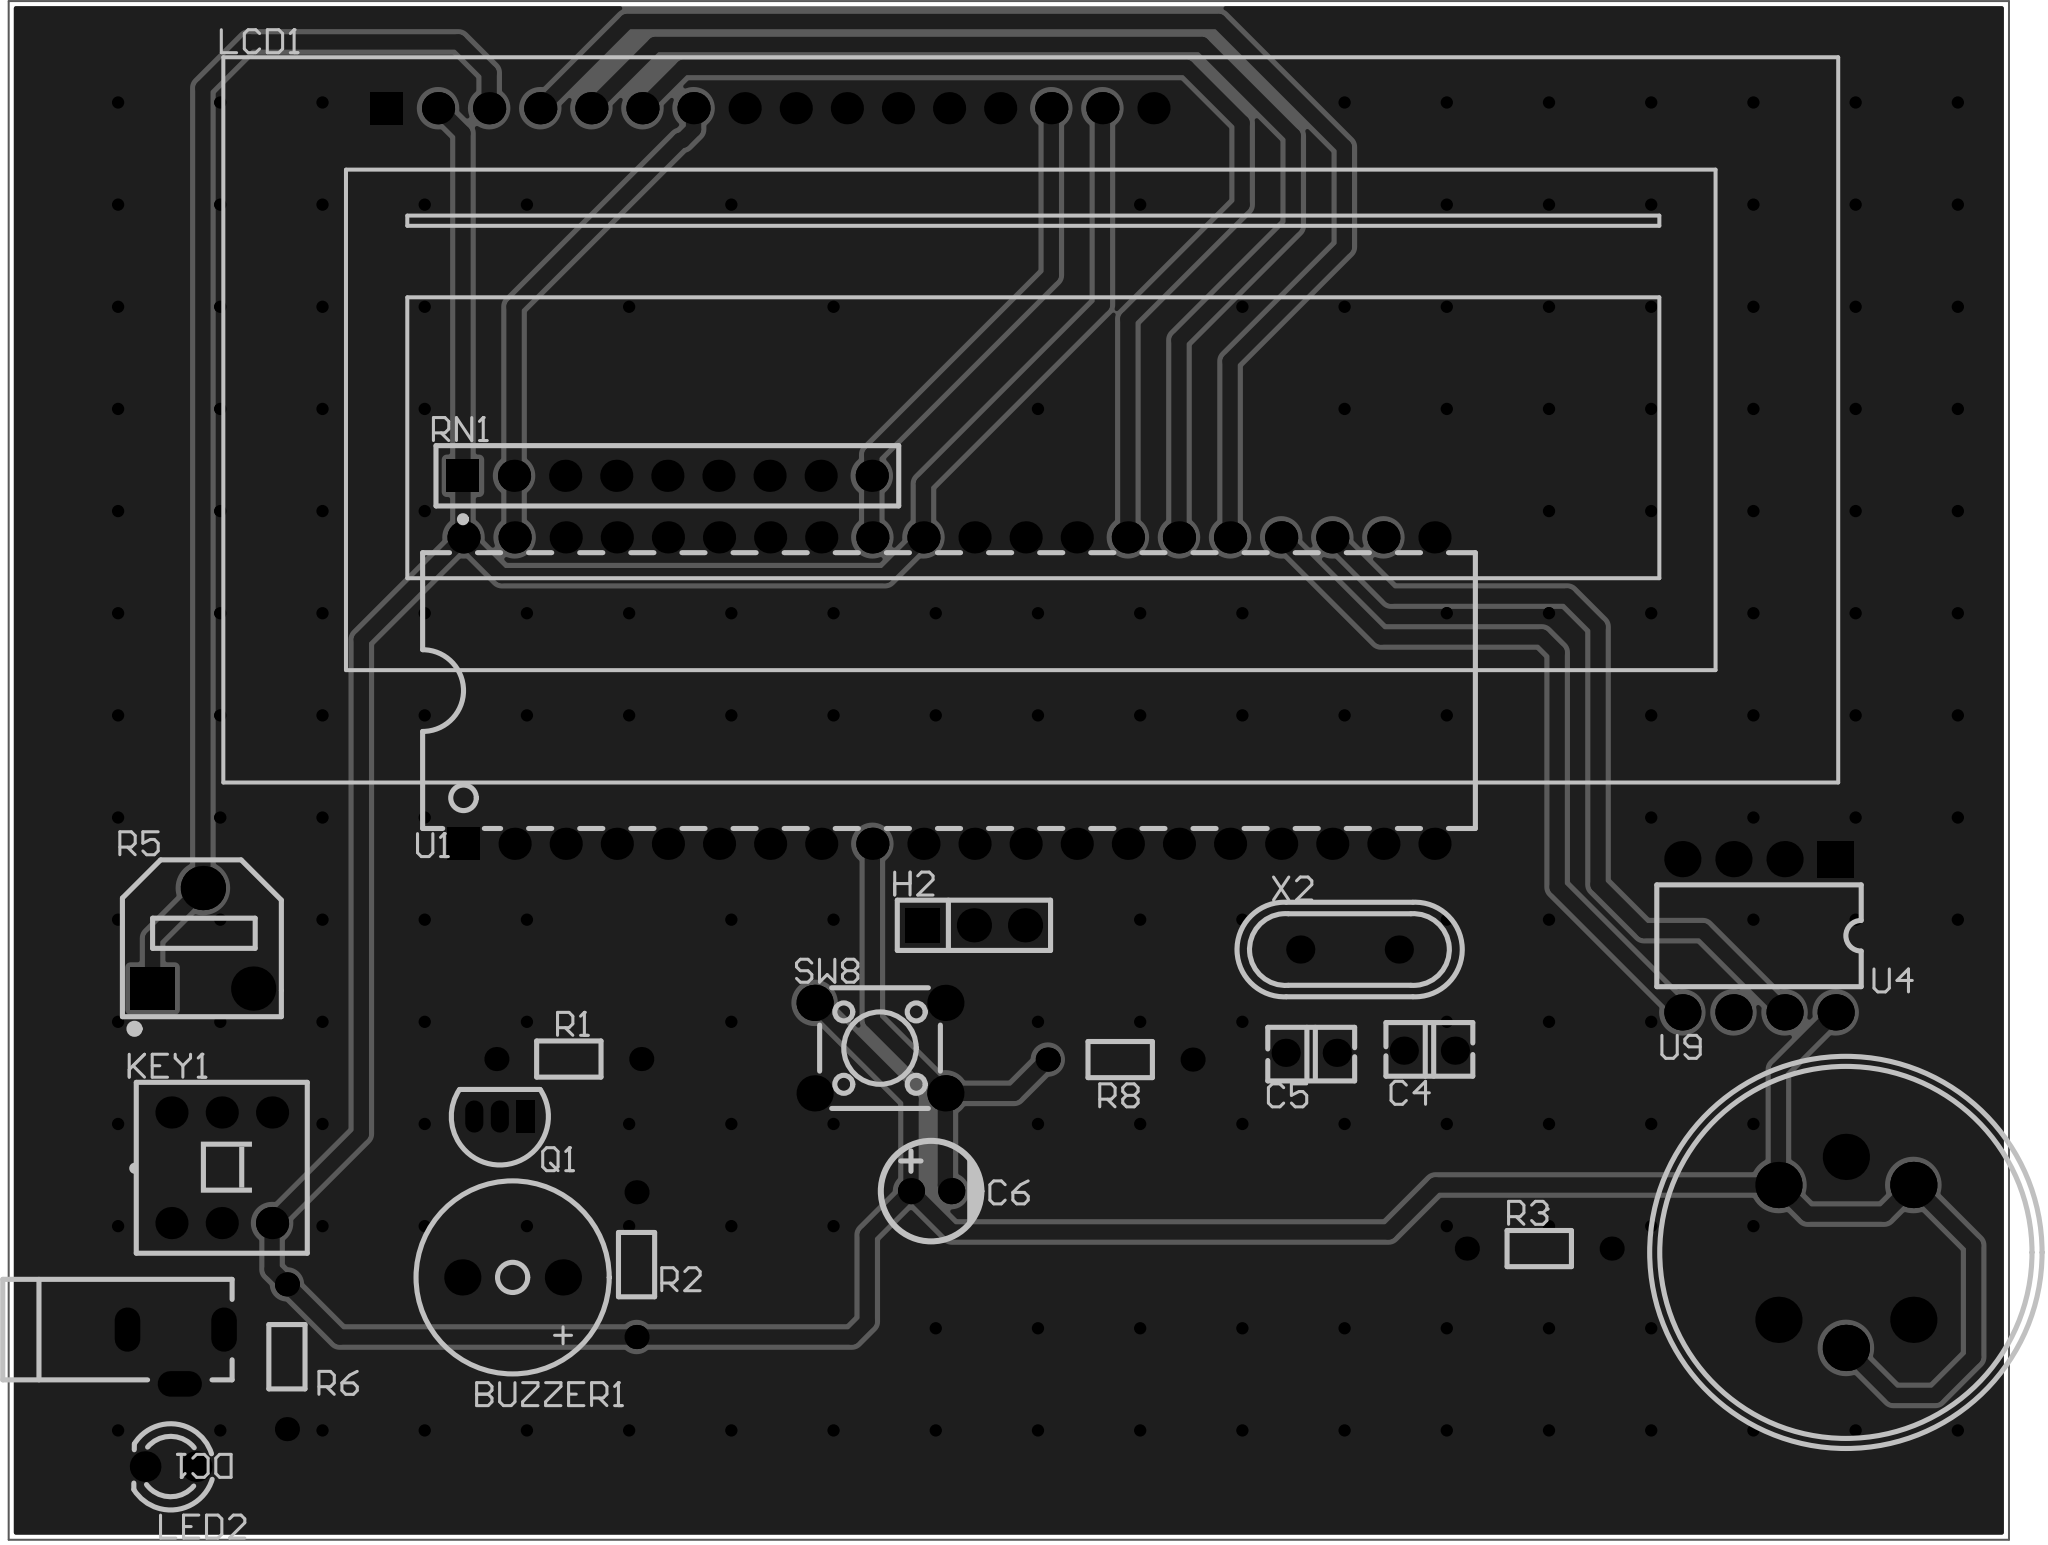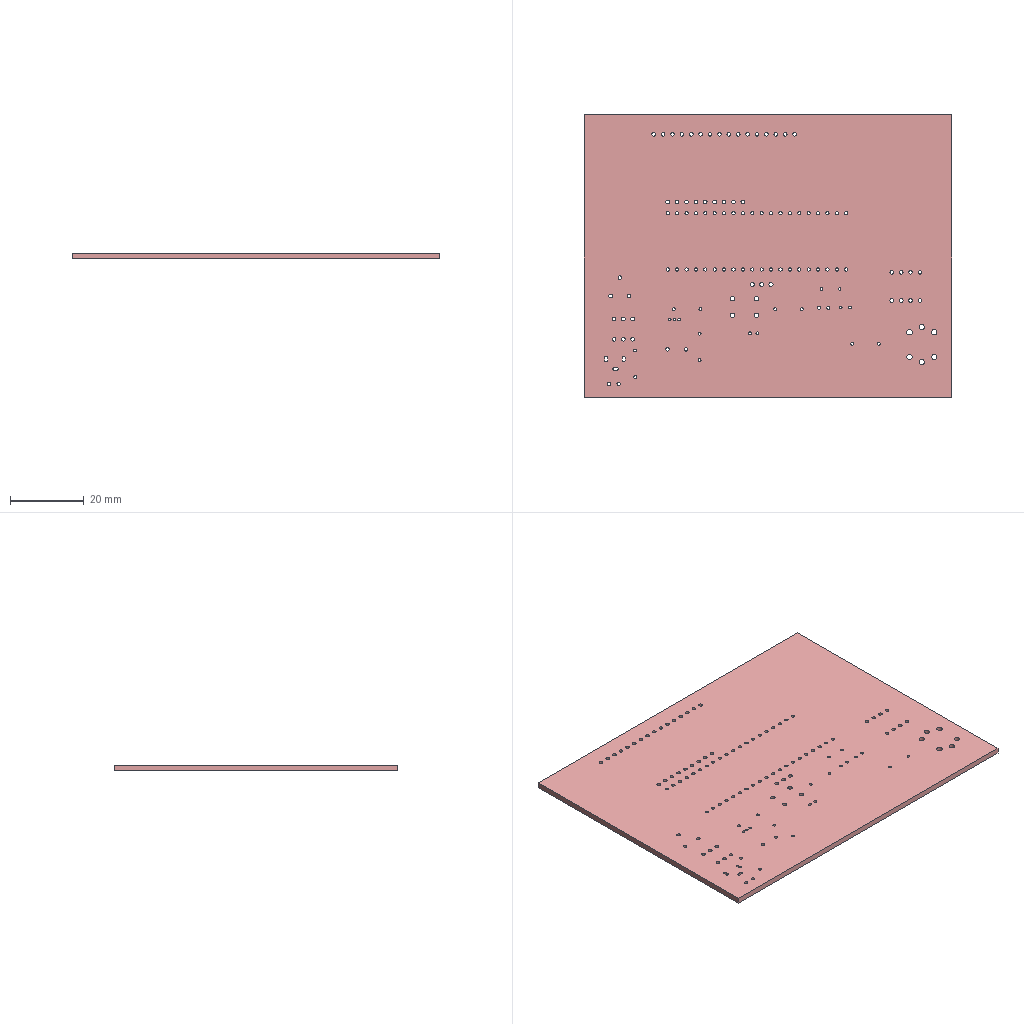Circuit board layout | Altium Designer | box 99.4 x 76.5 x 1.6 mm
Layer stack:
# Altium Designer layer stack of  (unit mm; dielectric type: 0 none, 1 core, 2 prepreg, 3 surface material)
index,name,kind,layer,copper_thickness_mm,dielectric_type,dielectric_thickness_mm,dielectric_material,dielectric_constant
0,Top Paste Mask Layer,other,,,,,,
1,Top Silkscreen Layer,other,,,,,,
2,Top Solder Mask Layer,dielectric,,,3,0.01,,3.3
3,Top Layer,copper,Top Layer,0.035,,,,
4,Dielectric1,dielectric,,,3,1.51,FR4,4.5
5,Bottom Layer,copper,Bottom Layer,0.035,,,,
6,Bottom Solder Mask Layer,dielectric,,,3,0.01,,3.3
7,Bottom Silkscreen Layer,other,,,,,,
8,Bottom Paste Mask Layer,other,,,,,,
# drill layer pairs: low layer,high layer
drill_pair,Top Layer,Bottom Layer
Part placement:
Designator,Comment,Layer,Footprint,Center-X(mm),Center-Y(mm),Rotation
C4,30pF,TopLayer,CAP-TH_L3.8-W2.5-P2.54-D0.50,162.052,107.061,180
C5,30pF,TopLayer,CAP-TH_L3.8-W2.5-P2.54-D0.50,156.18,106.952,0
C6,10uF,TopLayer,CAP-TH_BD5.0-P2.00-D0.8-FD-10UF50VC110GL,137.287,100.076,0
H2,,TopLayer,HDR-TH_3P-P2.54-V-M,139.416,113.296,0
KEY1,Non-latching switch 8.5×8.5 silent,TopLayer,SW-TH_6P-L8.5-W8.5-P2.54,102.031,101.237,0
LCD1,LCD1602,TopLayer,LCD1602,129.29,153.93,0
LED2,,TopLayer,LED_TH-3mm,99.491,86.378,180
R8,10kΩ,TopLayer,Res_1/8W,146.685,106.617,180
R5,10kΩ,TopLayer,RES-ADJ-SMD_RM065-V1,101.092,112.649,0
R6,1kΩ,TopLayer,Res_1/8W,105.27,91.839,90
SW8,,TopLayer,SW-TH_4P-L6.0-W6.0-P4.50-LS6.5,134.747,107.188,0
U1,STC89C52RC-40I-PDIP40,TopLayer,DIP-40_L52.0-W13.7-P2.54-LS15.2-BL,138.176,124.968,0
X2,11.059MHz,TopLayer,OSC-TH_L11.1-W4.7-P4.88,158.085,112.091,0
DC1,DC-002,TopLayer,DC-IN-TH_DC-3510,99.745,91.839,180
BUZZER1,3kHz,TopLayer,BUZ-TH_BD9.6-P5.00-D0.7-FD,116.487,95.785,180
RN1,-,TopLayer,RES-ARRAY-TH_9P-P2.54-D1.0,124.178,135.649,0
U4,XPT2046,TopLayer,DIP-8_L9.7-W6.4-P2.54-LS7.6-BL,178.435,112.776,180
U9,MQ-5,TopLayer,SENSOR-TH_MQ-5,182.753,97.028,0
Q1,,TopLayer,S8050_TO_92,115.852,103.786,180
R1,1K,TopLayer,Res_1/8W,119.281,106.644,180
R2,10kΩ,TopLayer,Res_1/8W,122.647,96.42,90
R3,5kΩ,TopLayer,Res_1/8W,167.513,97.218,0
Pad and via stacks:
# Altium Designer via and pad stacks of  (unit mm). Each distinct definition once, with the count of objects using it.
# via: kind,start_layer,end_layer,hole_mm,diameter_mm,mode(0 simple;1 top-mid-bottom;2 full stack),diameter_per_layer,count,example_net
# pad: kind,layer,hole_mm,hole_type(0 round;1 square;2 slot),plating,top_size,top_shape(1 round;2 rect;3 octagon;9 rounded rect),mid_size,bottom_size,mode,footprint,size_per_layer,count,example
pad,Multi-Layer,0.8,0,plated,1.4x1.4,1,1.4x1.4,1.4x1.4,0,CAP-TH_L3.8-W2.5-P2.54-D0.50,,4,C4.1
pad,Multi-Layer,0.8,0,plated,1.3x1.3,1,1.3x1.3,1.3x1.3,0,CAP-TH_BD5.0-P2.00-D0.8-FD-10UF50VC110GL,,2,C6.2
pad,Multi-Layer,1.1,0,plated,1.7x1.7,2,1.7x1.7,1.7x1.7,0,HDR-TH_3P-P2.54-V-M,,1,H2.1
pad,Multi-Layer,1.1,0,plated,1.7x1.7,1,1.7x1.7,1.7x1.7,0,HDR-TH_3P-P2.54-V-M,,2,H2.2
pad,Multi-Layer,1,0,plated,1.6x1.6,1,1.6x1.6,1.6x1.6,0,SW-TH_6P-L8.5-W8.5-P2.54,,6,KEY1.4
pad,Multi-Layer,1,0,plated,1.6x1.6,1,1.6x1.6,1.6x1.6,0,LCD1602,,15,LCD1.16
pad,Multi-Layer,1,0,plated,1.6x1.6,2,1.6x1.6,1.6x1.6,0,LCD1602,,1,LCD1.1
pad,Multi-Layer,0.9144,0,plated,1.524x1.524,1,1.524x1.524,1.524x1.524,0,LED_TH-3mm,,2,LED2.1
pad,Multi-Layer,0.8001,0,plated,1.199x1.199,1,1.199x1.199,1.199x1.199,0,Res_1/8W,,10,R8.1
pad,Multi-Layer,1,0,plated,2.2x2.1,2,2.2x2.1,2.2x2.1,0,RES-ADJ-SMD_RM065-V1,,1,R5.1
pad,Multi-Layer,1,0,plated,2.2x2.2,1,2.2x2.2,2.2x2.2,0,RES-ADJ-SMD_RM065-V1,,2,R5.3
pad,Multi-Layer,1.2,0,plated,1.8x1.8,1,1.8x1.8,1.8x1.8,0,SW-TH_4P-L6.0-W6.0-P4.50-LS6.5,,4,SW8.1
pad,Multi-Layer,0.889,0,plated,1.6x1.6,1,1.6x1.6,1.6x1.6,0,DIP-40_L52.0-W13.7-P2.54-LS15.2-BL,,39,U1.31
pad,Multi-Layer,0.889,0,plated,1.6x1.6,2,1.6x1.6,1.6x1.6,0,DIP-40_L52.0-W13.7-P2.54-LS15.2-BL,,1,U1.1
pad,Multi-Layer,0.7,0,plated,1.4x1.4,1,1.4x1.4,1.4x1.4,0,OSC-TH_L11.1-W4.7-P4.88,,2,X2.1
pad,Multi-Layer,0.8,2,plated,2.2x1.27,1,2.2x1.27,2.2x1.27,0,DC-IN-TH_DC-3510,,3,DC1.3
pad,Multi-Layer,1,0,plated,1.8x1.8,1,1.8x1.8,1.8x1.8,0,BUZ-TH_BD9.6-P5.00-D0.7-FD,,2,BUZZER1.2
pad,Multi-Layer,1,0,plated,1.6x1.6,2,1.6x1.6,1.6x1.6,0,RES-ARRAY-TH_9P-P2.54-D1.0,,1,RN1.1
pad,Multi-Layer,1,0,plated,1.6x1.6,1,1.6x1.6,1.6x1.6,0,RES-ARRAY-TH_9P-P2.54-D1.0,,8,RN1.2
pad,Multi-Layer,1,0,plated,1.8x1.8,2,1.8x1.8,1.8x1.8,0,DIP-8_L9.7-W6.4-P2.54-LS7.6-BL,,1,U4.1
pad,Multi-Layer,1,0,plated,1.8x1.8,1,1.8x1.8,1.8x1.8,0,DIP-8_L9.7-W6.4-P2.54-LS7.6-BL,,7,U4.2
pad,Multi-Layer,1.5,0,plated,2.3x2.3,1,2.3x2.3,2.3x2.3,0,SENSOR-TH_MQ-5,,6,U9.1
pad,Multi-Layer,0.701,0,plated,0.8992x1.6,2,0.8992x1.6,0.8992x1.6,0,S8050_TO_92,,1,Q1.1
pad,Multi-Layer,0.701,0,plated,0.8992x1.6,1,0.8992x1.6,0.8992x1.6,0,S8050_TO_92,,2,Q1.2
via,Top Layer,Bottom Layer,0.3048,0.61,0,,180,GND
Copper pours:
name,layer,net,type(0 solid;1 hatched;2 none)
Top Layer-GND,Top Layer,GND,0
Bottom Layer-GND,Bottom Layer,GND,0
Design rules, without the lines most boards share:
# Altium Designer design rules of  (exported by Altium Designer, unit mm)
# columns: name | kind | enabled | priority | scope1 | scope2 | descriptor | typed fields (field=value)
creepage | 65 | enabled | 1 | All | All | Creepage Distance Constraint =(0mil) (All),(All) |
copperRegion | 20 | enabled | 1 | (InNet('GND')) | All | Polygon Connect Rule(Relief Connect )(Conductor Width=10mil) (Relief Angle=90 Angle) (Entries=4) (Air Gap Width=10mil) ((InNet('GND'))),(All) | connect_style(0=relief,1=direct,2=none)=0 relief_conductor_width=0.254 relief_entries=4